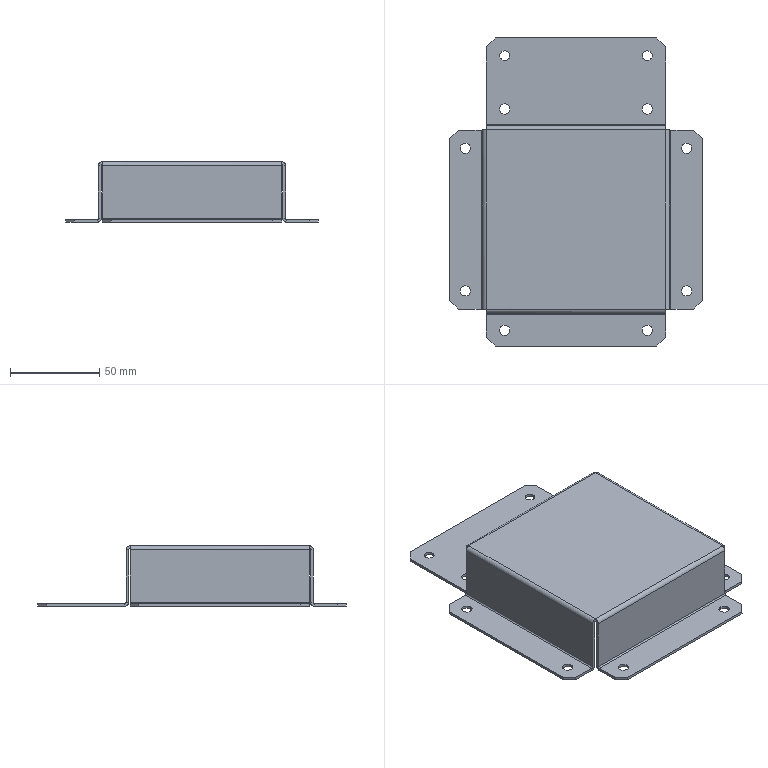Part | SolidWorks | features EdgeFlange 2, HoleWzd 2, BreakCorner 1, FlatPattern 1, MoveFace 1, SMBaseFlange 1, SheetMetal 1 | 1 solid | 98 faces | box 142 x 173 x 34 mm | volume 50656 mm3 | plane 54 | cylinder 36 | spline 8 | commonest cylinder face diameters 5.8 x16 1.473 x8 4.473 x8 5.5 x4